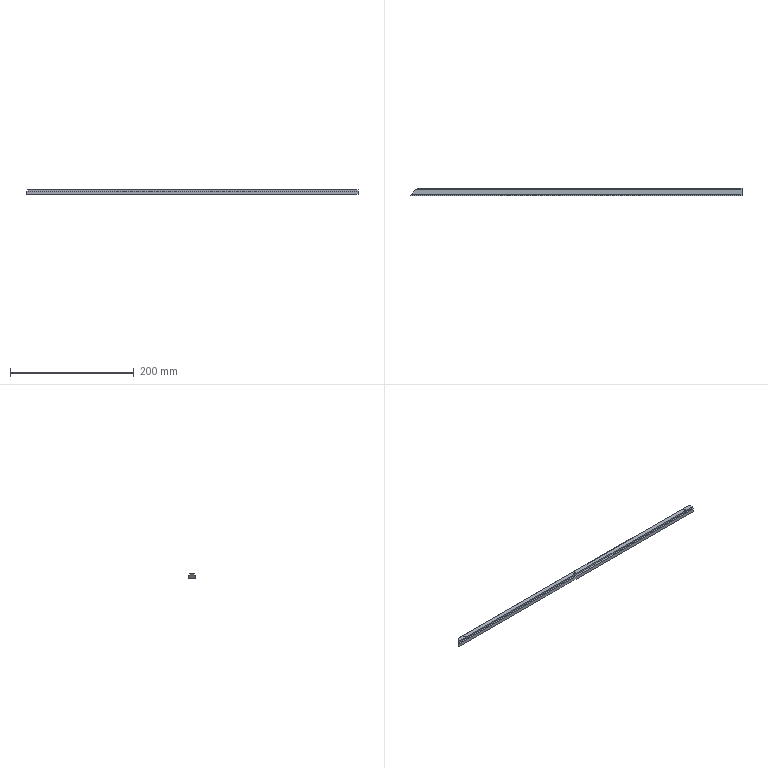Part | STEP file | J013-EBZ05-08-06 | 1 solid | 31 faces | box 535.5 x 12 x 8 mm | volume 43428 mm3 | plane 13 | cylinder 12 | cone 6 | commonest cylinder face diameters 3.24 x6 4 x6
STEP:
#1=CARTESIAN_POINT('',(15.,6.,7.835));
#2=VERTEX_POINT('',#1);
#3=CARTESIAN_POINT('',(16.62,6.,6.9));
#4=VERTEX_POINT('',#3);
#5=CARTESIAN_POINT('',(16.62,6.,6.9));
#6=DIRECTION('',(0.866,0.,-0.5));
#7=VECTOR('',#6,1000.);
#8=LINE('',#5,#7);
#9=EDGE_CURVE('',#2,#4,#8,.T.);
#10=ORIENTED_EDGE('',*,*,#9,.F.);
#11=CARTESIAN_POINT('',(13.38,6.,6.9));
#12=VERTEX_POINT('',#11);
#13=CARTESIAN_POINT('',(13.38,6.,6.9));
#14=DIRECTION('',(-0.866,0.,-0.5));
#15=VECTOR('',#14,1000.);
#16=LINE('',#13,#15);
#17=EDGE_CURVE('',#2,#12,#16,.T.);
#18=ORIENTED_EDGE('',*,*,#17,.T.);
#19=CARTESIAN_POINT('',(15.,6.,6.9));
#20=DIRECTION('',(0.,0.,-1.));
#21=DIRECTION('',(1.,0.,0.));
#22=AXIS2_PLACEMENT_3D('',#19,#20,#21);
#23=CIRCLE('',#22,1.62);
#24=EDGE_CURVE('',#12,#4,#23,.T.);
#25=ORIENTED_EDGE('',*,*,#24,.T.);
#26=EDGE_LOOP('',(#10,#18,#25));
#27=FACE_OUTER_BOUND('',#26,.T.);
#28=CARTESIAN_POINT('',(15.,6.,6.9));
#29=DIRECTION('',(0.,0.,-1.));
#30=DIRECTION('',(1.,0.,0.));
#31=AXIS2_PLACEMENT_3D('',#28,#29,#30);
#32=CONICAL_SURFACE('',#31,1.62,1.047);
#33=ADVANCED_FACE('',(#27),#32,.F.);
#34=ORIENTED_EDGE('',*,*,#24,.F.);
#35=CARTESIAN_POINT('',(13.38,6.,6.));
#36=VERTEX_POINT('',#35);
#37=CARTESIAN_POINT('',(13.38,6.,0.));
#38=DIRECTION('',(0.,0.,-1.));
#39=VECTOR('',#38,1000.);
#40=LINE('',#37,#39);
#41=EDGE_CURVE('',#12,#36,#40,.T.);
#42=ORIENTED_EDGE('',*,*,#41,.T.);
#43=CARTESIAN_POINT('',(16.62,6.,6.));
#44=VERTEX_POINT('',#43);
#45=CARTESIAN_POINT('',(15.,6.,6.));
#46=DIRECTION('',(0.,0.,-1.));
#47=DIRECTION('',(1.,0.,0.));
#48=AXIS2_PLACEMENT_3D('',#45,#46,#47);
#49=CIRCLE('',#48,1.62);
#50=EDGE_CURVE('',#36,#44,#49,.T.);
#51=ORIENTED_EDGE('',*,*,#50,.T.);
#52=CARTESIAN_POINT('',(16.62,6.,0.));
#53=DIRECTION('',(0.,0.,-1.));
#54=VECTOR('',#53,1000.);
#55=LINE('',#52,#54);
#56=EDGE_CURVE('',#4,#44,#55,.T.);
#57=ORIENTED_EDGE('',*,*,#56,.F.);
#58=EDGE_LOOP('',(#34,#42,#51,#57));
#59=FACE_OUTER_BOUND('',#58,.T.);
#60=CARTESIAN_POINT('',(15.,6.,0.));
#61=DIRECTION('',(0.,0.,-1.));
#62=DIRECTION('',(1.,0.,0.));
#63=AXIS2_PLACEMENT_3D('',#60,#61,#62);
#64=CYLINDRICAL_SURFACE('',#63,1.62);
#65=ADVANCED_FACE('',(#59),#64,.F.);
#66=CARTESIAN_POINT('',(13.,6.,6.));
#67=VERTEX_POINT('',#66);
#68=CARTESIAN_POINT('',(17.,6.,6.));
#69=VERTEX_POINT('',#68);
#70=CARTESIAN_POINT('',(15.,6.,6.));
#71=DIRECTION('',(0.,0.,-1.));
#72=DIRECTION('',(1.,0.,0.));
#73=AXIS2_PLACEMENT_3D('',#70,#71,#72);
#74=CIRCLE('',#73,2.);
#75=EDGE_CURVE('',#67,#69,#74,.T.);
#76=ORIENTED_EDGE('',*,*,#75,.F.);
#77=CARTESIAN_POINT('',(13.,6.,0.));
#78=VERTEX_POINT('',#77);
#79=CARTESIAN_POINT('',(13.,6.,0.));
#80=DIRECTION('',(0.,0.,-1.));
#81=VECTOR('',#80,1000.);
#82=LINE('',#79,#81);
#83=EDGE_CURVE('',#67,#78,#82,.T.);
#84=ORIENTED_EDGE('',*,*,#83,.T.);
#85=CARTESIAN_POINT('',(17.,6.,0.));
#86=VERTEX_POINT('',#85);
#87=CARTESIAN_POINT('',(15.,6.,0.));
#88=DIRECTION('',(0.,0.,-1.));
#89=DIRECTION('',(1.,0.,0.));
#90=AXIS2_PLACEMENT_3D('',#87,#88,#89);
#91=CIRCLE('',#90,2.);
#92=EDGE_CURVE('',#78,#86,#91,.T.);
#93=ORIENTED_EDGE('',*,*,#92,.T.);
#94=CARTESIAN_POINT('',(17.,6.,0.));
#95=DIRECTION('',(0.,0.,-1.));
#96=VECTOR('',#95,1000.);
#97=LINE('',#94,#96);
#98=EDGE_CURVE('',#69,#86,#97,.T.);
#99=ORIENTED_EDGE('',*,*,#98,.F.);
#100=EDGE_LOOP('',(#76,#84,#93,#99));
#101=FACE_OUTER_BOUND('',#100,.T.);
#102=CARTESIAN_POINT('',(15.,6.,0.));
#103=DIRECTION('',(0.,0.,-1.));
#104=DIRECTION('',(1.,0.,0.));
#105=AXIS2_PLACEMENT_3D('',#102,#103,#104);
#106=CYLINDRICAL_SURFACE('',#105,2.);
#107=ADVANCED_FACE('',(#101),#106,.F.);
#108=CARTESIAN_POINT('',(265.,6.,7.835));
#109=VERTEX_POINT('',#108);
#110=CARTESIAN_POINT('',(266.62,6.,6.9));
#111=VERTEX_POINT('',#110);
#112=CARTESIAN_POINT('',(266.62,6.,6.9));
#113=DIRECTION('',(0.866,0.,-0.5));
#114=VECTOR('',#113,1000.);
#115=LINE('',#112,#114);
#116=EDGE_CURVE('',#109,#111,#115,.T.);
#117=ORIENTED_EDGE('',*,*,#116,.F.);
#118=CARTESIAN_POINT('',(263.38,6.,6.9));
#119=VERTEX_POINT('',#118);
#120=CARTESIAN_POINT('',(263.38,6.,6.9));
#121=DIRECTION('',(-0.866,0.,-0.5));
#122=VECTOR('',#121,1000.);
#123=LINE('',#120,#122);
#124=EDGE_CURVE('',#109,#119,#123,.T.);
#125=ORIENTED_EDGE('',*,*,#124,.T.);
#126=CARTESIAN_POINT('',(265.,6.,6.9));
#127=DIRECTION('',(0.,0.,-1.));
#128=DIRECTION('',(1.,0.,0.));
#129=AXIS2_PLACEMENT_3D('',#126,#127,#128);
#130=CIRCLE('',#129,1.62);
#131=EDGE_CURVE('',#119,#111,#130,.T.);
#132=ORIENTED_EDGE('',*,*,#131,.T.);
#133=EDGE_LOOP('',(#117,#125,#132));
#134=FACE_OUTER_BOUND('',#133,.T.);
#135=CARTESIAN_POINT('',(265.,6.,6.9));
#136=DIRECTION('',(0.,0.,-1.));
#137=DIRECTION('',(1.,0.,0.));
#138=AXIS2_PLACEMENT_3D('',#135,#136,#137);
#139=CONICAL_SURFACE('',#138,1.62,1.047);
#140=ADVANCED_FACE('',(#134),#139,.F.);
#141=ORIENTED_EDGE('',*,*,#131,.F.);
#142=CARTESIAN_POINT('',(263.38,6.,6.));
#143=VERTEX_POINT('',#142);
#144=CARTESIAN_POINT('',(263.38,6.,0.));
#145=DIRECTION('',(0.,0.,-1.));
#146=VECTOR('',#145,1000.);
#147=LINE('',#144,#146);
#148=EDGE_CURVE('',#119,#143,#147,.T.);
#149=ORIENTED_EDGE('',*,*,#148,.T.);
#150=CARTESIAN_POINT('',(266.62,6.,6.));
#151=VERTEX_POINT('',#150);
#152=CARTESIAN_POINT('',(265.,6.,6.));
#153=DIRECTION('',(0.,0.,-1.));
#154=DIRECTION('',(1.,0.,0.));
#155=AXIS2_PLACEMENT_3D('',#152,#153,#154);
#156=CIRCLE('',#155,1.62);
#157=EDGE_CURVE('',#143,#151,#156,.T.);
#158=ORIENTED_EDGE('',*,*,#157,.T.);
#159=CARTESIAN_POINT('',(266.62,6.,0.));
#160=DIRECTION('',(0.,0.,-1.));
#161=VECTOR('',#160,1000.);
#162=LINE('',#159,#161);
#163=EDGE_CURVE('',#111,#151,#162,.T.);
#164=ORIENTED_EDGE('',*,*,#163,.F.);
#165=EDGE_LOOP('',(#141,#149,#158,#164));
#166=FACE_OUTER_BOUND('',#165,.T.);
#167=CARTESIAN_POINT('',(265.,6.,0.));
#168=DIRECTION('',(0.,0.,-1.));
#169=DIRECTION('',(1.,0.,0.));
#170=AXIS2_PLACEMENT_3D('',#167,#168,#169);
#171=CYLINDRICAL_SURFACE('',#170,1.62);
#172=ADVANCED_FACE('',(#166),#171,.F.);
#173=CARTESIAN_POINT('',(263.,6.,6.));
#174=VERTEX_POINT('',#173);
#175=CARTESIAN_POINT('',(267.,6.,6.));
#176=VERTEX_POINT('',#175);
#177=CARTESIAN_POINT('',(265.,6.,6.));
#178=DIRECTION('',(0.,0.,-1.));
#179=DIRECTION('',(1.,0.,0.));
#180=AXIS2_PLACEMENT_3D('',#177,#178,#179);
#181=CIRCLE('',#180,2.);
#182=EDGE_CURVE('',#174,#176,#181,.T.);
#183=ORIENTED_EDGE('',*,*,#182,.F.);
#184=CARTESIAN_POINT('',(263.,6.,0.));
#185=VERTEX_POINT('',#184);
#186=CARTESIAN_POINT('',(263.,6.,0.));
#187=DIRECTION('',(0.,0.,-1.));
#188=VECTOR('',#187,1000.);
#189=LINE('',#186,#188);
#190=EDGE_CURVE('',#174,#185,#189,.T.);
#191=ORIENTED_EDGE('',*,*,#190,.T.);
#192=CARTESIAN_POINT('',(267.,6.,0.));
#193=VERTEX_POINT('',#192);
#194=CARTESIAN_POINT('',(265.,6.,0.));
#195=DIRECTION('',(0.,0.,-1.));
#196=DIRECTION('',(1.,0.,0.));
#197=AXIS2_PLACEMENT_3D('',#194,#195,#196);
#198=CIRCLE('',#197,2.);
#199=EDGE_CURVE('',#185,#193,#198,.T.);
#200=ORIENTED_EDGE('',*,*,#199,.T.);
#201=CARTESIAN_POINT('',(267.,6.,0.));
#202=DIRECTION('',(0.,0.,-1.));
#203=VECTOR('',#202,1000.);
#204=LINE('',#201,#203);
#205=EDGE_CURVE('',#176,#193,#204,.T.);
#206=ORIENTED_EDGE('',*,*,#205,.F.);
#207=EDGE_LOOP('',(#183,#191,#200,#206));
#208=FACE_OUTER_BOUND('',#207,.T.);
#209=CARTESIAN_POINT('',(265.,6.,0.));
#210=DIRECTION('',(0.,0.,-1.));
#211=DIRECTION('',(1.,0.,0.));
#212=AXIS2_PLACEMENT_3D('',#209,#210,#211);
#213=CYLINDRICAL_SURFACE('',#212,2.);
#214=ADVANCED_FACE('',(#208),#213,.F.);
#215=CARTESIAN_POINT('',(515.,6.,7.835));
#216=VERTEX_POINT('',#215);
#217=CARTESIAN_POINT('',(516.62,6.,6.9));
#218=VERTEX_POINT('',#217);
#219=CARTESIAN_POINT('',(516.62,6.,6.9));
#220=DIRECTION('',(0.866,0.,-0.5));
#221=VECTOR('',#220,1000.);
#222=LINE('',#219,#221);
#223=EDGE_CURVE('',#216,#218,#222,.T.);
#224=ORIENTED_EDGE('',*,*,#223,.F.);
#225=CARTESIAN_POINT('',(513.38,6.,6.9));
#226=VERTEX_POINT('',#225);
#227=CARTESIAN_POINT('',(513.38,6.,6.9));
#228=DIRECTION('',(-0.866,0.,-0.5));
#229=VECTOR('',#228,1000.);
#230=LINE('',#227,#229);
#231=EDGE_CURVE('',#216,#226,#230,.T.);
#232=ORIENTED_EDGE('',*,*,#231,.T.);
#233=CARTESIAN_POINT('',(515.,6.,6.9));
#234=DIRECTION('',(0.,0.,-1.));
#235=DIRECTION('',(1.,0.,0.));
#236=AXIS2_PLACEMENT_3D('',#233,#234,#235);
#237=CIRCLE('',#236,1.62);
#238=EDGE_CURVE('',#226,#218,#237,.T.);
#239=ORIENTED_EDGE('',*,*,#238,.T.);
#240=EDGE_LOOP('',(#224,#232,#239));
#241=FACE_OUTER_BOUND('',#240,.T.);
#242=CARTESIAN_POINT('',(515.,6.,6.9));
#243=DIRECTION('',(0.,0.,-1.));
#244=DIRECTION('',(1.,0.,0.));
#245=AXIS2_PLACEMENT_3D('',#242,#243,#244);
#246=CONICAL_SURFACE('',#245,1.62,1.047);
#247=ADVANCED_FACE('',(#241),#246,.F.);
#248=ORIENTED_EDGE('',*,*,#238,.F.);
#249=CARTESIAN_POINT('',(513.38,6.,6.));
#250=VERTEX_POINT('',#249);
#251=CARTESIAN_POINT('',(513.38,6.,0.));
#252=DIRECTION('',(0.,0.,-1.));
#253=VECTOR('',#252,1000.);
#254=LINE('',#251,#253);
#255=EDGE_CURVE('',#226,#250,#254,.T.);
#256=ORIENTED_EDGE('',*,*,#255,.T.);
#257=CARTESIAN_POINT('',(516.62,6.,6.));
#258=VERTEX_POINT('',#257);
#259=CARTESIAN_POINT('',(515.,6.,6.));
#260=DIRECTION('',(0.,0.,-1.));
#261=DIRECTION('',(1.,0.,0.));
#262=AXIS2_PLACEMENT_3D('',#259,#260,#261);
#263=CIRCLE('',#262,1.62);
#264=EDGE_CURVE('',#250,#258,#263,.T.);
#265=ORIENTED_EDGE('',*,*,#264,.T.);
#266=CARTESIAN_POINT('',(516.62,6.,0.));
#267=DIRECTION('',(0.,0.,-1.));
#268=VECTOR('',#267,1000.);
#269=LINE('',#266,#268);
#270=EDGE_CURVE('',#218,#258,#269,.T.);
#271=ORIENTED_EDGE('',*,*,#270,.F.);
#272=EDGE_LOOP('',(#248,#256,#265,#271));
#273=FACE_OUTER_BOUND('',#272,.T.);
#274=CARTESIAN_POINT('',(515.,6.,0.));
#275=DIRECTION('',(0.,0.,-1.));
#276=DIRECTION('',(1.,0.,0.));
#277=AXIS2_PLACEMENT_3D('',#274,#275,#276);
#278=CYLINDRICAL_SURFACE('',#277,1.62);
#279=ADVANCED_FACE('',(#273),#278,.F.);
#280=CARTESIAN_POINT('',(513.,6.,6.));
#281=VERTEX_POINT('',#280);
#282=CARTESIAN_POINT('',(517.,6.,6.));
#283=VERTEX_POINT('',#282);
#284=CARTESIAN_POINT('',(515.,6.,6.));
#285=DIRECTION('',(0.,0.,-1.));
#286=DIRECTION('',(1.,0.,0.));
#287=AXIS2_PLACEMENT_3D('',#284,#285,#286);
#288=CIRCLE('',#287,2.);
#289=EDGE_CURVE('',#281,#283,#288,.T.);
#290=ORIENTED_EDGE('',*,*,#289,.F.);
#291=CARTESIAN_POINT('',(513.,6.,0.));
#292=VERTEX_POINT('',#291);
#293=CARTESIAN_POINT('',(513.,6.,0.));
#294=DIRECTION('',(0.,0.,-1.));
#295=VECTOR('',#294,1000.);
#296=LINE('',#293,#295);
#297=EDGE_CURVE('',#281,#292,#296,.T.);
#298=ORIENTED_EDGE('',*,*,#297,.T.);
#299=CARTESIAN_POINT('',(517.,6.,0.));
#300=VERTEX_POINT('',#299);
#301=CARTESIAN_POINT('',(515.,6.,0.));
#302=DIRECTION('',(0.,0.,-1.));
#303=DIRECTION('',(1.,0.,0.));
#304=AXIS2_PLACEMENT_3D('',#301,#302,#303);
#305=CIRCLE('',#304,2.);
#306=EDGE_CURVE('',#292,#300,#305,.T.);
#307=ORIENTED_EDGE('',*,*,#306,.T.);
#308=CARTESIAN_POINT('',(517.,6.,0.));
#309=DIRECTION('',(0.,0.,-1.));
#310=VECTOR('',#309,1000.);
#311=LINE('',#308,#310);
#312=EDGE_CURVE('',#283,#300,#311,.T.);
#313=ORIENTED_EDGE('',*,*,#312,.F.);
#314=EDGE_LOOP('',(#290,#298,#307,#313));
#315=FACE_OUTER_BOUND('',#314,.T.);
#316=CARTESIAN_POINT('',(515.,6.,0.));
#317=DIRECTION('',(0.,0.,-1.));
#318=DIRECTION('',(1.,0.,0.));
#319=AXIS2_PLACEMENT_3D('',#316,#317,#318);
#320=CYLINDRICAL_SURFACE('',#319,2.);
#321=ADVANCED_FACE('',(#315),#320,.F.);
#322=CARTESIAN_POINT('',(6.5,12.,5.5));
#323=VERTEX_POINT('',#322);
#324=CARTESIAN_POINT('',(530.,12.,5.5));
#325=VERTEX_POINT('',#324);
#326=CARTESIAN_POINT('',(-5.5,12.,5.5));
#327=DIRECTION('',(1.,0.,0.));
#328=VECTOR('',#327,1000.);
#329=LINE('',#326,#328);
#330=EDGE_CURVE('',#323,#325,#329,.T.);
#331=ORIENTED_EDGE('',*,*,#330,.F.);
#332=CARTESIAN_POINT('',(3.8,9.3,5.5));
#333=VERTEX_POINT('',#332);
#334=CARTESIAN_POINT('',(-900.891,-895.391,5.5));
#335=DIRECTION('',(-0.7071,-0.7071,0.));
#336=VECTOR('',#335,1000.);
#337=LINE('',#334,#336);
#338=EDGE_CURVE('',#323,#333,#337,.T.);
#339=ORIENTED_EDGE('',*,*,#338,.T.);
#340=CARTESIAN_POINT('',(530.,9.3,5.5));
#341=VERTEX_POINT('',#340);
#342=CARTESIAN_POINT('',(-5.5,9.3,5.5));
#343=DIRECTION('',(1.,0.,0.));
#344=VECTOR('',#343,1000.);
#345=LINE('',#342,#344);
#346=EDGE_CURVE('',#333,#341,#345,.T.);
#347=ORIENTED_EDGE('',*,*,#346,.T.);
#348=CARTESIAN_POINT('',(530.,12.,5.5));
#349=DIRECTION('',(0.,-1.,0.));
#350=VECTOR('',#349,1000.);
#351=LINE('',#348,#350);
#352=EDGE_CURVE('',#325,#341,#351,.T.);
#353=ORIENTED_EDGE('',*,*,#352,.F.);
#354=EDGE_LOOP('',(#331,#339,#347,#353));
#355=FACE_OUTER_BOUND('',#354,.T.);
#356=CARTESIAN_POINT('',(-581.652,-1214.63,5.5));
#357=DIRECTION('',(0.,0.,-1.));
#358=DIRECTION('',(1.,0.,0.));
#359=AXIS2_PLACEMENT_3D('',#356,#357,#358);
#360=PLANE('',#359);
#361=ADVANCED_FACE('',(#355),#360,.F.);
#362=CARTESIAN_POINT('',(530.,0.,5.5));
#363=VERTEX_POINT('',#362);
#364=CARTESIAN_POINT('',(-5.5,0.,5.5));
#365=VERTEX_POINT('',#364);
#366=CARTESIAN_POINT('',(530.,0.,5.5));
#367=DIRECTION('',(-1.,0.,0.));
#368=VECTOR('',#367,1000.);
#369=LINE('',#366,#368);
#370=EDGE_CURVE('',#363,#365,#369,.T.);
#371=ORIENTED_EDGE('',*,*,#370,.T.);
#372=CARTESIAN_POINT('',(-5.5,0.,0.));
#373=VERTEX_POINT('',#372);
#374=CARTESIAN_POINT('',(-5.5,0.,0.));
#375=DIRECTION('',(0.,0.,1.));
#376=VECTOR('',#375,1000.);
#377=LINE('',#374,#376);
#378=EDGE_CURVE('',#373,#365,#377,.T.);
#379=ORIENTED_EDGE('',*,*,#378,.F.);
#380=CARTESIAN_POINT('',(530.,0.,0.));
#381=VERTEX_POINT('',#380);
#382=CARTESIAN_POINT('',(530.,0.,0.));
#383=DIRECTION('',(-1.,0.,0.));
#384=VECTOR('',#383,1000.);
#385=LINE('',#382,#384);
#386=EDGE_CURVE('',#381,#373,#385,.T.);
#387=ORIENTED_EDGE('',*,*,#386,.F.);
#388=CARTESIAN_POINT('',(530.,0.,0.));
#389=DIRECTION('',(0.,0.,1.));
#390=VECTOR('',#389,1000.);
#391=LINE('',#388,#390);
#392=EDGE_CURVE('',#381,#363,#391,.T.);
#393=ORIENTED_EDGE('',*,*,#392,.T.);
#394=EDGE_LOOP('',(#371,#379,#387,#393));
#395=FACE_OUTER_BOUND('',#394,.T.);
#396=CARTESIAN_POINT('',(530.,0.,0.));
#397=DIRECTION('',(0.,1.,0.));
#398=DIRECTION('',(0.,0.,1.));
#399=AXIS2_PLACEMENT_3D('',#396,#397,#398);
#400=PLANE('',#399);
#401=ADVANCED_FACE('',(#395),#400,.F.);
#402=CARTESIAN_POINT('',(6.5,12.,0.));
#403=VERTEX_POINT('',#402);
#404=CARTESIAN_POINT('',(530.,12.,0.));
#405=VERTEX_POINT('',#404);
#406=CARTESIAN_POINT('',(-5.5,12.,0.));
#407=DIRECTION('',(1.,0.,0.));
#408=VECTOR('',#407,1000.);
#409=LINE('',#406,#408);
#410=EDGE_CURVE('',#403,#405,#409,.T.);
#411=ORIENTED_EDGE('',*,*,#410,.F.);
#412=CARTESIAN_POINT('',(6.5,12.,-0.001006));
#413=DIRECTION('',(0.,0.,1.));
#414=VECTOR('',#413,1000.);
#415=LINE('',#412,#414);
#416=EDGE_CURVE('',#403,#323,#415,.T.);
#417=ORIENTED_EDGE('',*,*,#416,.T.);
#418=ORIENTED_EDGE('',*,*,#330,.T.);
#419=CARTESIAN_POINT('',(530.,12.,0.));
#420=DIRECTION('',(0.,0.,1.));
#421=VECTOR('',#420,1000.);
#422=LINE('',#419,#421);
#423=EDGE_CURVE('',#405,#325,#422,.T.);
#424=ORIENTED_EDGE('',*,*,#423,.F.);
#425=EDGE_LOOP('',(#411,#417,#418,#424));
#426=FACE_OUTER_BOUND('',#425,.T.);
#427=CARTESIAN_POINT('',(-5.5,12.,0.));
#428=DIRECTION('',(0.,-1.,0.));
#429=DIRECTION('',(0.,0.,-1.));
#430=AXIS2_PLACEMENT_3D('',#427,#428,#429);
#431=PLANE('',#430);
#432=ADVANCED_FACE('',(#426),#431,.F.);
#433=ORIENTED_EDGE('',*,*,#352,.T.);
#434=CARTESIAN_POINT('',(530.,9.3,8.));
#435=VERTEX_POINT('',#434);
#436=CARTESIAN_POINT('',(530.,9.3,8.));
#437=DIRECTION('',(0.,0.,-1.));
#438=VECTOR('',#437,1000.);
#439=LINE('',#436,#438);
#440=EDGE_CURVE('',#435,#341,#439,.T.);
#441=ORIENTED_EDGE('',*,*,#440,.F.);
#442=CARTESIAN_POINT('',(530.,2.7,8.));
#443=VERTEX_POINT('',#442);
#444=CARTESIAN_POINT('',(530.,9.3,8.));
#445=DIRECTION('',(0.,-1.,0.));
#446=VECTOR('',#445,1000.);
#447=LINE('',#444,#446);
#448=EDGE_CURVE('',#435,#443,#447,.T.);
#449=ORIENTED_EDGE('',*,*,#448,.T.);
#450=CARTESIAN_POINT('',(530.,2.7,5.5));
#451=VERTEX_POINT('',#450);
#452=CARTESIAN_POINT('',(530.,2.7,8.));
#453=DIRECTION('',(0.,0.,-1.));
#454=VECTOR('',#453,1000.);
#455=LINE('',#452,#454);
#456=EDGE_CURVE('',#443,#451,#455,.T.);
#457=ORIENTED_EDGE('',*,*,#456,.T.);
#458=CARTESIAN_POINT('',(530.,12.,5.5));
#459=DIRECTION('',(0.,-1.,0.));
#460=VECTOR('',#459,1000.);
#461=LINE('',#458,#460);
#462=EDGE_CURVE('',#451,#363,#461,.T.);
#463=ORIENTED_EDGE('',*,*,#462,.T.);
#464=ORIENTED_EDGE('',*,*,#392,.F.);
#465=CARTESIAN_POINT('',(530.,12.,0.));
#466=DIRECTION('',(0.,-1.,0.));
#467=VECTOR('',#466,1000.);
#468=LINE('',#465,#467);
#469=EDGE_CURVE('',#405,#381,#468,.T.);
#470=ORIENTED_EDGE('',*,*,#469,.F.);
#471=ORIENTED_EDGE('',*,*,#423,.T.);
#472=EDGE_LOOP('',(#433,#441,#449,#457,#463,#464,#470,#471));
#473=FACE_OUTER_BOUND('',#472,.T.);
#474=CARTESIAN_POINT('',(530.,12.,0.));
#475=DIRECTION('',(-1.,0.,0.));
#476=DIRECTION('',(0.,0.,-1.));
#477=AXIS2_PLACEMENT_3D('',#474,#475,#476);
#478=PLANE('',#477);
#479=ADVANCED_FACE('',(#473),#478,.F.);
#480=CARTESIAN_POINT('',(-900.891,-895.391,0.));
#481=DIRECTION('',(-0.7071,-0.7071,0.));
#482=VECTOR('',#481,1000.);
#483=LINE('',#480,#482);
#484=EDGE_CURVE('',#403,#373,#483,.T.);
#485=ORIENTED_EDGE('',*,*,#484,.F.);
#486=ORIENTED_EDGE('',*,*,#410,.T.);
#487=ORIENTED_EDGE('',*,*,#469,.T.);
#488=ORIENTED_EDGE('',*,*,#386,.T.);
#489=EDGE_LOOP('',(#485,#486,#487,#488));
#490=FACE_OUTER_BOUND('',#489,.T.);
#491=CARTESIAN_POINT('',(15.,6.,0.));
#492=DIRECTION('',(0.,0.,-1.));
#493=DIRECTION('',(1.,0.,0.));
#494=AXIS2_PLACEMENT_3D('',#491,#492,#493);
#495=CIRCLE('',#494,2.);
#496=EDGE_CURVE('',#86,#78,#495,.T.);
#497=ORIENTED_EDGE('',*,*,#496,.F.);
#498=ORIENTED_EDGE('',*,*,#92,.F.);
#499=EDGE_LOOP('',(#497,#498));
#500=FACE_BOUND('',#499,.T.);
#501=CARTESIAN_POINT('',(265.,6.,0.));
#502=DIRECTION('',(0.,0.,-1.));
#503=DIRECTION('',(1.,0.,0.));
#504=AXIS2_PLACEMENT_3D('',#501,#502,#503);
#505=CIRCLE('',#504,2.);
#506=EDGE_CURVE('',#193,#185,#505,.T.);
#507=ORIENTED_EDGE('',*,*,#506,.F.);
#508=ORIENTED_EDGE('',*,*,#199,.F.);
#509=EDGE_LOOP('',(#507,#508));
#510=FACE_BOUND('',#509,.T.);
#511=CARTESIAN_POINT('',(515.,6.,0.));
#512=DIRECTION('',(0.,0.,-1.));
#513=DIRECTION('',(1.,0.,0.));
#514=AXIS2_PLACEMENT_3D('',#511,#512,#513);
#515=CIRCLE('',#514,2.);
#516=EDGE_CURVE('',#300,#292,#515,.T.);
#517=ORIENTED_EDGE('',*,*,#516,.F.);
#518=ORIENTED_EDGE('',*,*,#306,.F.);
#519=EDGE_LOOP('',(#517,#518));
#520=FACE_BOUND('',#519,.T.);
#521=CARTESIAN_POINT('',(-581.652,-1214.63,0.));
#522=DIRECTION('',(0.,0.,-1.));
#523=DIRECTION('',(1.,0.,0.));
#524=AXIS2_PLACEMENT_3D('',#521,#522,#523);
#525=PLANE('',#524);
#526=ADVANCED_FACE('',(#490,#500,#510,#520),#525,.T.);
#527=CARTESIAN_POINT('',(-2.8,2.7,5.5));
#528=VERTEX_POINT('',#527);
#529=CARTESIAN_POINT('',(530.,2.7,5.5));
#530=DIRECTION('',(-1.,0.,0.));
#531=VECTOR('',#530,1000.);
#532=LINE('',#529,#531);
#533=EDGE_CURVE('',#451,#528,#532,.T.);
#534=ORIENTED_EDGE('',*,*,#533,.T.);
#535=CARTESIAN_POINT('',(-900.891,-895.391,5.5));
#536=DIRECTION('',(-0.7071,-0.7071,0.));
#537=VECTOR('',#536,1000.);
#538=LINE('',#535,#537);
#539=EDGE_CURVE('',#528,#365,#538,.T.);
#540=ORIENTED_EDGE('',*,*,#539,.T.);
#541=ORIENTED_EDGE('',*,*,#370,.F.);
#542=ORIENTED_EDGE('',*,*,#462,.F.);
#543=EDGE_LOOP('',(#534,#540,#541,#542));
#544=FACE_OUTER_BOUND('',#543,.T.);
#545=CARTESIAN_POINT('',(-581.652,-1214.63,5.5));
#546=DIRECTION('',(0.,0.,-1.));
#547=DIRECTION('',(1.,0.,0.));
#548=AXIS2_PLACEMENT_3D('',#545,#546,#547);
#549=PLANE('',#548);
#550=ADVANCED_FACE('',(#544),#549,.F.);
#551=CARTESIAN_POINT('',(3.8,9.3,8.));
#552=VERTEX_POINT('',#551);
#553=CARTESIAN_POINT('',(3.8,9.3,8.));
#554=DIRECTION('',(0.,0.,-1.));
#555=VECTOR('',#554,1000.);
#556=LINE('',#553,#555);
#557=EDGE_CURVE('',#552,#333,#556,.T.);
#558=ORIENTED_EDGE('',*,*,#557,.F.);
#559=CARTESIAN_POINT('',(-5.5,9.3,8.));
#560=DIRECTION('',(1.,0.,0.));
#561=VECTOR('',#560,1000.);
#562=LINE('',#559,#561);
#563=EDGE_CURVE('',#552,#435,#562,.T.);
#564=ORIENTED_EDGE('',*,*,#563,.T.);
#565=ORIENTED_EDGE('',*,*,#440,.T.);
#566=ORIENTED_EDGE('',*,*,#346,.F.);
#567=EDGE_LOOP('',(#558,#564,#565,#566));
#568=FACE_OUTER_BOUND('',#567,.T.);
#569=CARTESIAN_POINT('',(-5.5,9.3,8.));
#570=DIRECTION('',(0.,1.,0.));
#571=DIRECTION('',(0.,0.,1.));
#572=AXIS2_PLACEMENT_3D('',#569,#570,#571);
#573=PLANE('',#572);
#574=ADVANCED_FACE('',(#568),#573,.T.);
#575=CARTESIAN_POINT('',(-2.8,2.7,8.));
#576=VERTEX_POINT('',#575);
#577=CARTESIAN_POINT('',(-2.8,2.7,8.));
#578=DIRECTION('',(0.,0.,1.));
#579=VECTOR('',#578,1000.);
#580=LINE('',#577,#579);
#581=EDGE_CURVE('',#528,#576,#580,.T.);
#582=ORIENTED_EDGE('',*,*,#581,.F.);
#583=ORIENTED_EDGE('',*,*,#533,.F.);
#584=ORIENTED_EDGE('',*,*,#456,.F.);
#585=CARTESIAN_POINT('',(530.,2.7,8.));
#586=DIRECTION('',(-1.,0.,0.));
#587=VECTOR('',#586,1000.);
#588=LINE('',#585,#587);
#589=EDGE_CURVE('',#443,#576,#588,.T.);
#590=ORIENTED_EDGE('',*,*,#589,.T.);
#591=EDGE_LOOP('',(#582,#583,#584,#590));
#592=FACE_OUTER_BOUND('',#591,.T.);
#593=CARTESIAN_POINT('',(530.,2.7,8.));
#594=DIRECTION('',(0.,-1.,0.));
#595=DIRECTION('',(0.,0.,-1.));
#596=AXIS2_PLACEMENT_3D('',#593,#594,#595);
#597=PLANE('',#596);
#598=ADVANCED_FACE('',(#592),#597,.T.);
#599=ORIENTED_EDGE('',*,*,#563,.F.);
#600=CARTESIAN_POINT('',(-900.891,-895.391,8.));
#601=DIRECTION('',(-0.7071,-0.7071,0.));
#602=VECTOR('',#601,1000.);
#603=LINE('',#600,#602);
#604=EDGE_CURVE('',#552,#576,#603,.T.);
#605=ORIENTED_EDGE('',*,*,#604,.T.);
#606=ORIENTED_EDGE('',*,*,#589,.F.);
#607=ORIENTED_EDGE('',*,*,#448,.F.);
#608=EDGE_LOOP('',(#599,#605,#606,#607));
#609=FACE_OUTER_BOUND('',#608,.T.);
#610=CARTESIAN_POINT('',(-581.652,-1214.629,8.));
#611=DIRECTION('',(0.,0.,-1.));
#612=DIRECTION('',(1.,0.,0.));
#613=AXIS2_PLACEMENT_3D('',#610,#611,#612);
#614=PLANE('',#613);
#615=ADVANCED_FACE('',(#609),#614,.F.);
#616=ORIENTED_EDGE('',*,*,#297,.F.);
#617=CARTESIAN_POINT('',(515.,6.,6.));
#618=DIRECTION('',(0.,0.,-1.));
#619=DIRECTION('',(1.,0.,0.));
#620=AXIS2_PLACEMENT_3D('',#617,#618,#619);
#621=CIRCLE('',#620,2.);
#622=EDGE_CURVE('',#283,#281,#621,.T.);
#623=ORIENTED_EDGE('',*,*,#622,.F.);
#624=ORIENTED_EDGE('',*,*,#312,.T.);
#625=ORIENTED_EDGE('',*,*,#516,.T.);
#626=EDGE_LOOP('',(#616,#623,#624,#625));
#627=FACE_OUTER_BOUND('',#626,.T.);
#628=CARTESIAN_POINT('',(515.,6.,0.));
#629=DIRECTION('',(0.,0.,-1.));
#630=DIRECTION('',(1.,0.,0.));
#631=AXIS2_PLACEMENT_3D('',#628,#629,#630);
#632=CYLINDRICAL_SURFACE('',#631,2.);
#633=ADVANCED_FACE('',(#627),#632,.F.);
#634=CARTESIAN_POINT('',(515.,6.,6.));
#635=DIRECTION('',(0.,0.,-1.));
#636=DIRECTION('',(1.,0.,0.));
#637=AXIS2_PLACEMENT_3D('',#634,#635,#636);
#638=CIRCLE('',#637,1.62);
#639=EDGE_CURVE('',#258,#250,#638,.T.);
#640=ORIENTED_EDGE('',*,*,#639,.F.);
#641=ORIENTED_EDGE('',*,*,#264,.F.);
#642=EDGE_LOOP('',(#640,#641));
#643=FACE_BOUND('',#642,.T.);
#644=ORIENTED_EDGE('',*,*,#622,.T.);
#645=ORIENTED_EDGE('',*,*,#289,.T.);
#646=EDGE_LOOP('',(#644,#645));
#647=FACE_OUTER_BOUND('',#646,.T.);
#648=CARTESIAN_POINT('',(513.,6.,6.));
#649=DIRECTION('',(0.,0.,1.));
#650=DIRECTION('',(-1.,0.,0.));
#651=AXIS2_PLACEMENT_3D('',#648,#649,#650);
#652=PLANE('',#651);
#653=ADVANCED_FACE('',(#643,#647),#652,.F.);
#654=ORIENTED_EDGE('',*,*,#255,.F.);
#655=CARTESIAN_POINT('',(515.,6.,6.9));
#656=DIRECTION('',(0.,0.,-1.));
#657=DIRECTION('',(1.,0.,0.));
#658=AXIS2_PLACEMENT_3D('',#655,#656,#657);
#659=CIRCLE('',#658,1.62);
#660=EDGE_CURVE('',#218,#226,#659,.T.);
#661=ORIENTED_EDGE('',*,*,#660,.F.);
#662=ORIENTED_EDGE('',*,*,#270,.T.);
#663=ORIENTED_EDGE('',*,*,#639,.T.);
#664=EDGE_LOOP('',(#654,#661,#662,#663));
#665=FACE_OUTER_BOUND('',#664,.T.);
#666=CARTESIAN_POINT('',(515.,6.,0.));
#667=DIRECTION('',(0.,0.,-1.));
#668=DIRECTION('',(1.,0.,0.));
#669=AXIS2_PLACEMENT_3D('',#666,#667,#668);
#670=CYLINDRICAL_SURFACE('',#669,1.62);
#671=ADVANCED_FACE('',(#665),#670,.F.);
#672=ORIENTED_EDGE('',*,*,#231,.F.);
#673=ORIENTED_EDGE('',*,*,#223,.T.);
#674=ORIENTED_EDGE('',*,*,#660,.T.);
#675=EDGE_LOOP('',(#672,#673,#674));
#676=FACE_OUTER_BOUND('',#675,.T.);
#677=CARTESIAN_POINT('',(515.,6.,6.9));
#678=DIRECTION('',(0.,0.,-1.));
#679=DIRECTION('',(1.,0.,0.));
#680=AXIS2_PLACEMENT_3D('',#677,#678,#679);
#681=CONICAL_SURFACE('',#680,1.62,1.047);
#682=ADVANCED_FACE('',(#676),#681,.F.);
#683=ORIENTED_EDGE('',*,*,#190,.F.);
#684=CARTESIAN_POINT('',(265.,6.,6.));
#685=DIRECTION('',(0.,0.,-1.));
#686=DIRECTION('',(1.,0.,0.));
#687=AXIS2_PLACEMENT_3D('',#684,#685,#686);
#688=CIRCLE('',#687,2.);
#689=EDGE_CURVE('',#176,#174,#688,.T.);
#690=ORIENTED_EDGE('',*,*,#689,.F.);
#691=ORIENTED_EDGE('',*,*,#205,.T.);
#692=ORIENTED_EDGE('',*,*,#506,.T.);
#693=EDGE_LOOP('',(#683,#690,#691,#692));
#694=FACE_OUTER_BOUND('',#693,.T.);
#695=CARTESIAN_POINT('',(265.,6.,0.));
#696=DIRECTION('',(0.,0.,-1.));
#697=DIRECTION('',(1.,0.,0.));
#698=AXIS2_PLACEMENT_3D('',#695,#696,#697);
#699=CYLINDRICAL_SURFACE('',#698,2.);
#700=ADVANCED_FACE('',(#694),#699,.F.);
#701=CARTESIAN_POINT('',(265.,6.,6.));
#702=DIRECTION('',(0.,0.,-1.));
#703=DIRECTION('',(1.,0.,0.));
#704=AXIS2_PLACEMENT_3D('',#701,#702,#703);
#705=CIRCLE('',#704,1.62);
#706=EDGE_CURVE('',#151,#143,#705,.T.);
#707=ORIENTED_EDGE('',*,*,#706,.F.);
#708=ORIENTED_EDGE('',*,*,#157,.F.);
#709=EDGE_LOOP('',(#707,#708));
#710=FACE_BOUND('',#709,.T.);
#711=ORIENTED_EDGE('',*,*,#689,.T.);
#712=ORIENTED_EDGE('',*,*,#182,.T.);
#713=EDGE_LOOP('',(#711,#712));
#714=FACE_OUTER_BOUND('',#713,.T.);
#715=CARTESIAN_POINT('',(263.,6.,6.));
#716=DIRECTION('',(0.,0.,1.));
#717=DIRECTION('',(-1.,0.,0.));
#718=AXIS2_PLACEMENT_3D('',#715,#716,#717);
#719=PLANE('',#718);
#720=ADVANCED_FACE('',(#710,#714),#719,.F.);
#721=ORIENTED_EDGE('',*,*,#148,.F.);
#722=CARTESIAN_POINT('',(265.,6.,6.9));
#723=DIRECTION('',(0.,0.,-1.));
#724=DIRECTION('',(1.,0.,0.));
#725=AXIS2_PLACEMENT_3D('',#722,#723,#724);
#726=CIRCLE('',#725,1.62);
#727=EDGE_CURVE('',#111,#119,#726,.T.);
#728=ORIENTED_EDGE('',*,*,#727,.F.);
#729=ORIENTED_EDGE('',*,*,#163,.T.);
#730=ORIENTED_EDGE('',*,*,#706,.T.);
#731=EDGE_LOOP('',(#721,#728,#729,#730));
#732=FACE_OUTER_BOUND('',#731,.T.);
#733=CARTESIAN_POINT('',(265.,6.,0.));
#734=DIRECTION('',(0.,0.,-1.));
#735=DIRECTION('',(1.,0.,0.));
#736=AXIS2_PLACEMENT_3D('',#733,#734,#735);
#737=CYLINDRICAL_SURFACE('',#736,1.62);
#738=ADVANCED_FACE('',(#732),#737,.F.);
#739=ORIENTED_EDGE('',*,*,#124,.F.);
#740=ORIENTED_EDGE('',*,*,#116,.T.);
#741=ORIENTED_EDGE('',*,*,#727,.T.);
#742=EDGE_LOOP('',(#739,#740,#741));
#743=FACE_OUTER_BOUND('',#742,.T.);
#744=CARTESIAN_POINT('',(265.,6.,6.9));
#745=DIRECTION('',(0.,0.,-1.));
#746=DIRECTION('',(1.,0.,0.));
#747=AXIS2_PLACEMENT_3D('',#744,#745,#746);
#748=CONICAL_SURFACE('',#747,1.62,1.047);
#749=ADVANCED_FACE('',(#743),#748,.F.);
#750=ORIENTED_EDGE('',*,*,#83,.F.);
#751=CARTESIAN_POINT('',(15.,6.,6.));
#752=DIRECTION('',(0.,0.,-1.));
#753=DIRECTION('',(1.,0.,0.));
#754=AXIS2_PLACEMENT_3D('',#751,#752,#753);
#755=CIRCLE('',#754,2.);
#756=EDGE_CURVE('',#69,#67,#755,.T.);
#757=ORIENTED_EDGE('',*,*,#756,.F.);
#758=ORIENTED_EDGE('',*,*,#98,.T.);
#759=ORIENTED_EDGE('',*,*,#496,.T.);
#760=EDGE_LOOP('',(#750,#757,#758,#759));
#761=FACE_OUTER_BOUND('',#760,.T.);
#762=CARTESIAN_POINT('',(15.,6.,0.));
#763=DIRECTION('',(0.,0.,-1.));
#764=DIRECTION('',(1.,0.,0.));
#765=AXIS2_PLACEMENT_3D('',#762,#763,#764);
#766=CYLINDRICAL_SURFACE('',#765,2.);
#767=ADVANCED_FACE('',(#761),#766,.F.);
#768=CARTESIAN_POINT('',(15.,6.,6.));
#769=DIRECTION('',(0.,0.,-1.));
#770=DIRECTION('',(1.,0.,0.));
#771=AXIS2_PLACEMENT_3D('',#768,#769,#770);
#772=CIRCLE('',#771,1.62);
#773=EDGE_CURVE('',#44,#36,#772,.T.);
#774=ORIENTED_EDGE('',*,*,#773,.F.);
#775=ORIENTED_EDGE('',*,*,#50,.F.);
#776=EDGE_LOOP('',(#774,#775));
#777=FACE_BOUND('',#776,.T.);
#778=ORIENTED_EDGE('',*,*,#756,.T.);
#779=ORIENTED_EDGE('',*,*,#75,.T.);
#780=EDGE_LOOP('',(#778,#779));
#781=FACE_OUTER_BOUND('',#780,.T.);
#782=CARTESIAN_POINT('',(13.,6.,6.));
#783=DIRECTION('',(0.,0.,1.));
#784=DIRECTION('',(-1.,0.,0.));
#785=AXIS2_PLACEMENT_3D('',#782,#783,#784);
#786=PLANE('',#785);
#787=ADVANCED_FACE('',(#777,#781),#786,.F.);
#788=ORIENTED_EDGE('',*,*,#41,.F.);
#789=CARTESIAN_POINT('',(15.,6.,6.9));
#790=DIRECTION('',(0.,0.,-1.));
#791=DIRECTION('',(1.,0.,0.));
#792=AXIS2_PLACEMENT_3D('',#789,#790,#791);
#793=CIRCLE('',#792,1.62);
#794=EDGE_CURVE('',#4,#12,#793,.T.);
#795=ORIENTED_EDGE('',*,*,#794,.F.);
#796=ORIENTED_EDGE('',*,*,#56,.T.);
#797=ORIENTED_EDGE('',*,*,#773,.T.);
#798=EDGE_LOOP('',(#788,#795,#796,#797));
#799=FACE_OUTER_BOUND('',#798,.T.);
#800=CARTESIAN_POINT('',(15.,6.,0.));
#801=DIRECTION('',(0.,0.,-1.));
#802=DIRECTION('',(1.,0.,0.));
#803=AXIS2_PLACEMENT_3D('',#800,#801,#802);
#804=CYLINDRICAL_SURFACE('',#803,1.62);
#805=ADVANCED_FACE('',(#799),#804,.F.);
#806=ORIENTED_EDGE('',*,*,#17,.F.);
#807=ORIENTED_EDGE('',*,*,#9,.T.);
#808=ORIENTED_EDGE('',*,*,#794,.T.);
#809=EDGE_LOOP('',(#806,#807,#808));
#810=FACE_OUTER_BOUND('',#809,.T.);
#811=CARTESIAN_POINT('',(15.,6.,6.9));
#812=DIRECTION('',(0.,0.,-1.));
#813=DIRECTION('',(1.,0.,0.));
#814=AXIS2_PLACEMENT_3D('',#811,#812,#813);
#815=CONICAL_SURFACE('',#814,1.62,1.047);
#816=ADVANCED_FACE('',(#810),#815,.F.);
#817=ORIENTED_EDGE('',*,*,#416,.F.);
#818=ORIENTED_EDGE('',*,*,#484,.T.);
#819=ORIENTED_EDGE('',*,*,#378,.T.);
#820=ORIENTED_EDGE('',*,*,#539,.F.);
#821=ORIENTED_EDGE('',*,*,#581,.T.);
#822=ORIENTED_EDGE('',*,*,#604,.F.);
#823=ORIENTED_EDGE('',*,*,#557,.T.);
#824=ORIENTED_EDGE('',*,*,#338,.F.);
#825=EDGE_LOOP('',(#817,#818,#819,#820,#821,#822,#823,#824));
#826=FACE_OUTER_BOUND('',#825,.T.);
#827=CARTESIAN_POINT('',(-5.5,0.,-0.001006));
#828=DIRECTION('',(0.7071,-0.7071,0.));
#829=DIRECTION('',(0.7071,0.7071,0.));
#830=AXIS2_PLACEMENT_3D('',#827,#828,#829);
#831=PLANE('',#830);
#832=ADVANCED_FACE('',(#826),#831,.F.);
#833=CLOSED_SHELL('',(#33,#65,#107,#140,#172,#214,#247,#279,#321,#361,#401,#432,#479,#526,#550,#574,#598,#615,#633,#653,#671,#682,#700,#720,#738,#749,#767,#787,#805,#816,#832));
#834=MANIFOLD_SOLID_BREP('',#833);
#835=CARTESIAN_POINT('',(0.,0.,0.));
#836=DIRECTION('',(0.,0.,1.));
#837=DIRECTION('',(1.,0.,0.));
#838=AXIS2_PLACEMENT_3D('',#835,#836,#837);
#839=(LENGTH_UNIT()NAMED_UNIT(*)SI_UNIT(.MILLI.,.METRE.));
#840=UNCERTAINTY_MEASURE_WITH_UNIT(LENGTH_MEASURE(0.00001),#839,'','');
#841=(NAMED_UNIT(*)PLANE_ANGLE_UNIT()SI_UNIT($,.RADIAN.));
#842=(NAMED_UNIT(*)SI_UNIT($,.STERADIAN.)SOLID_ANGLE_UNIT());
#843=(GEOMETRIC_REPRESENTATION_CONTEXT(3)GLOBAL_UNCERTAINTY_ASSIGNED_CONTEXT((#840))GLOBAL_UNIT_ASSIGNED_CONTEXT((#839,#841,#842))REPRESENTATION_CONTEXT('',''));
#844=ADVANCED_BREP_SHAPE_REPRESENTATION('',(#834,#838),#843);